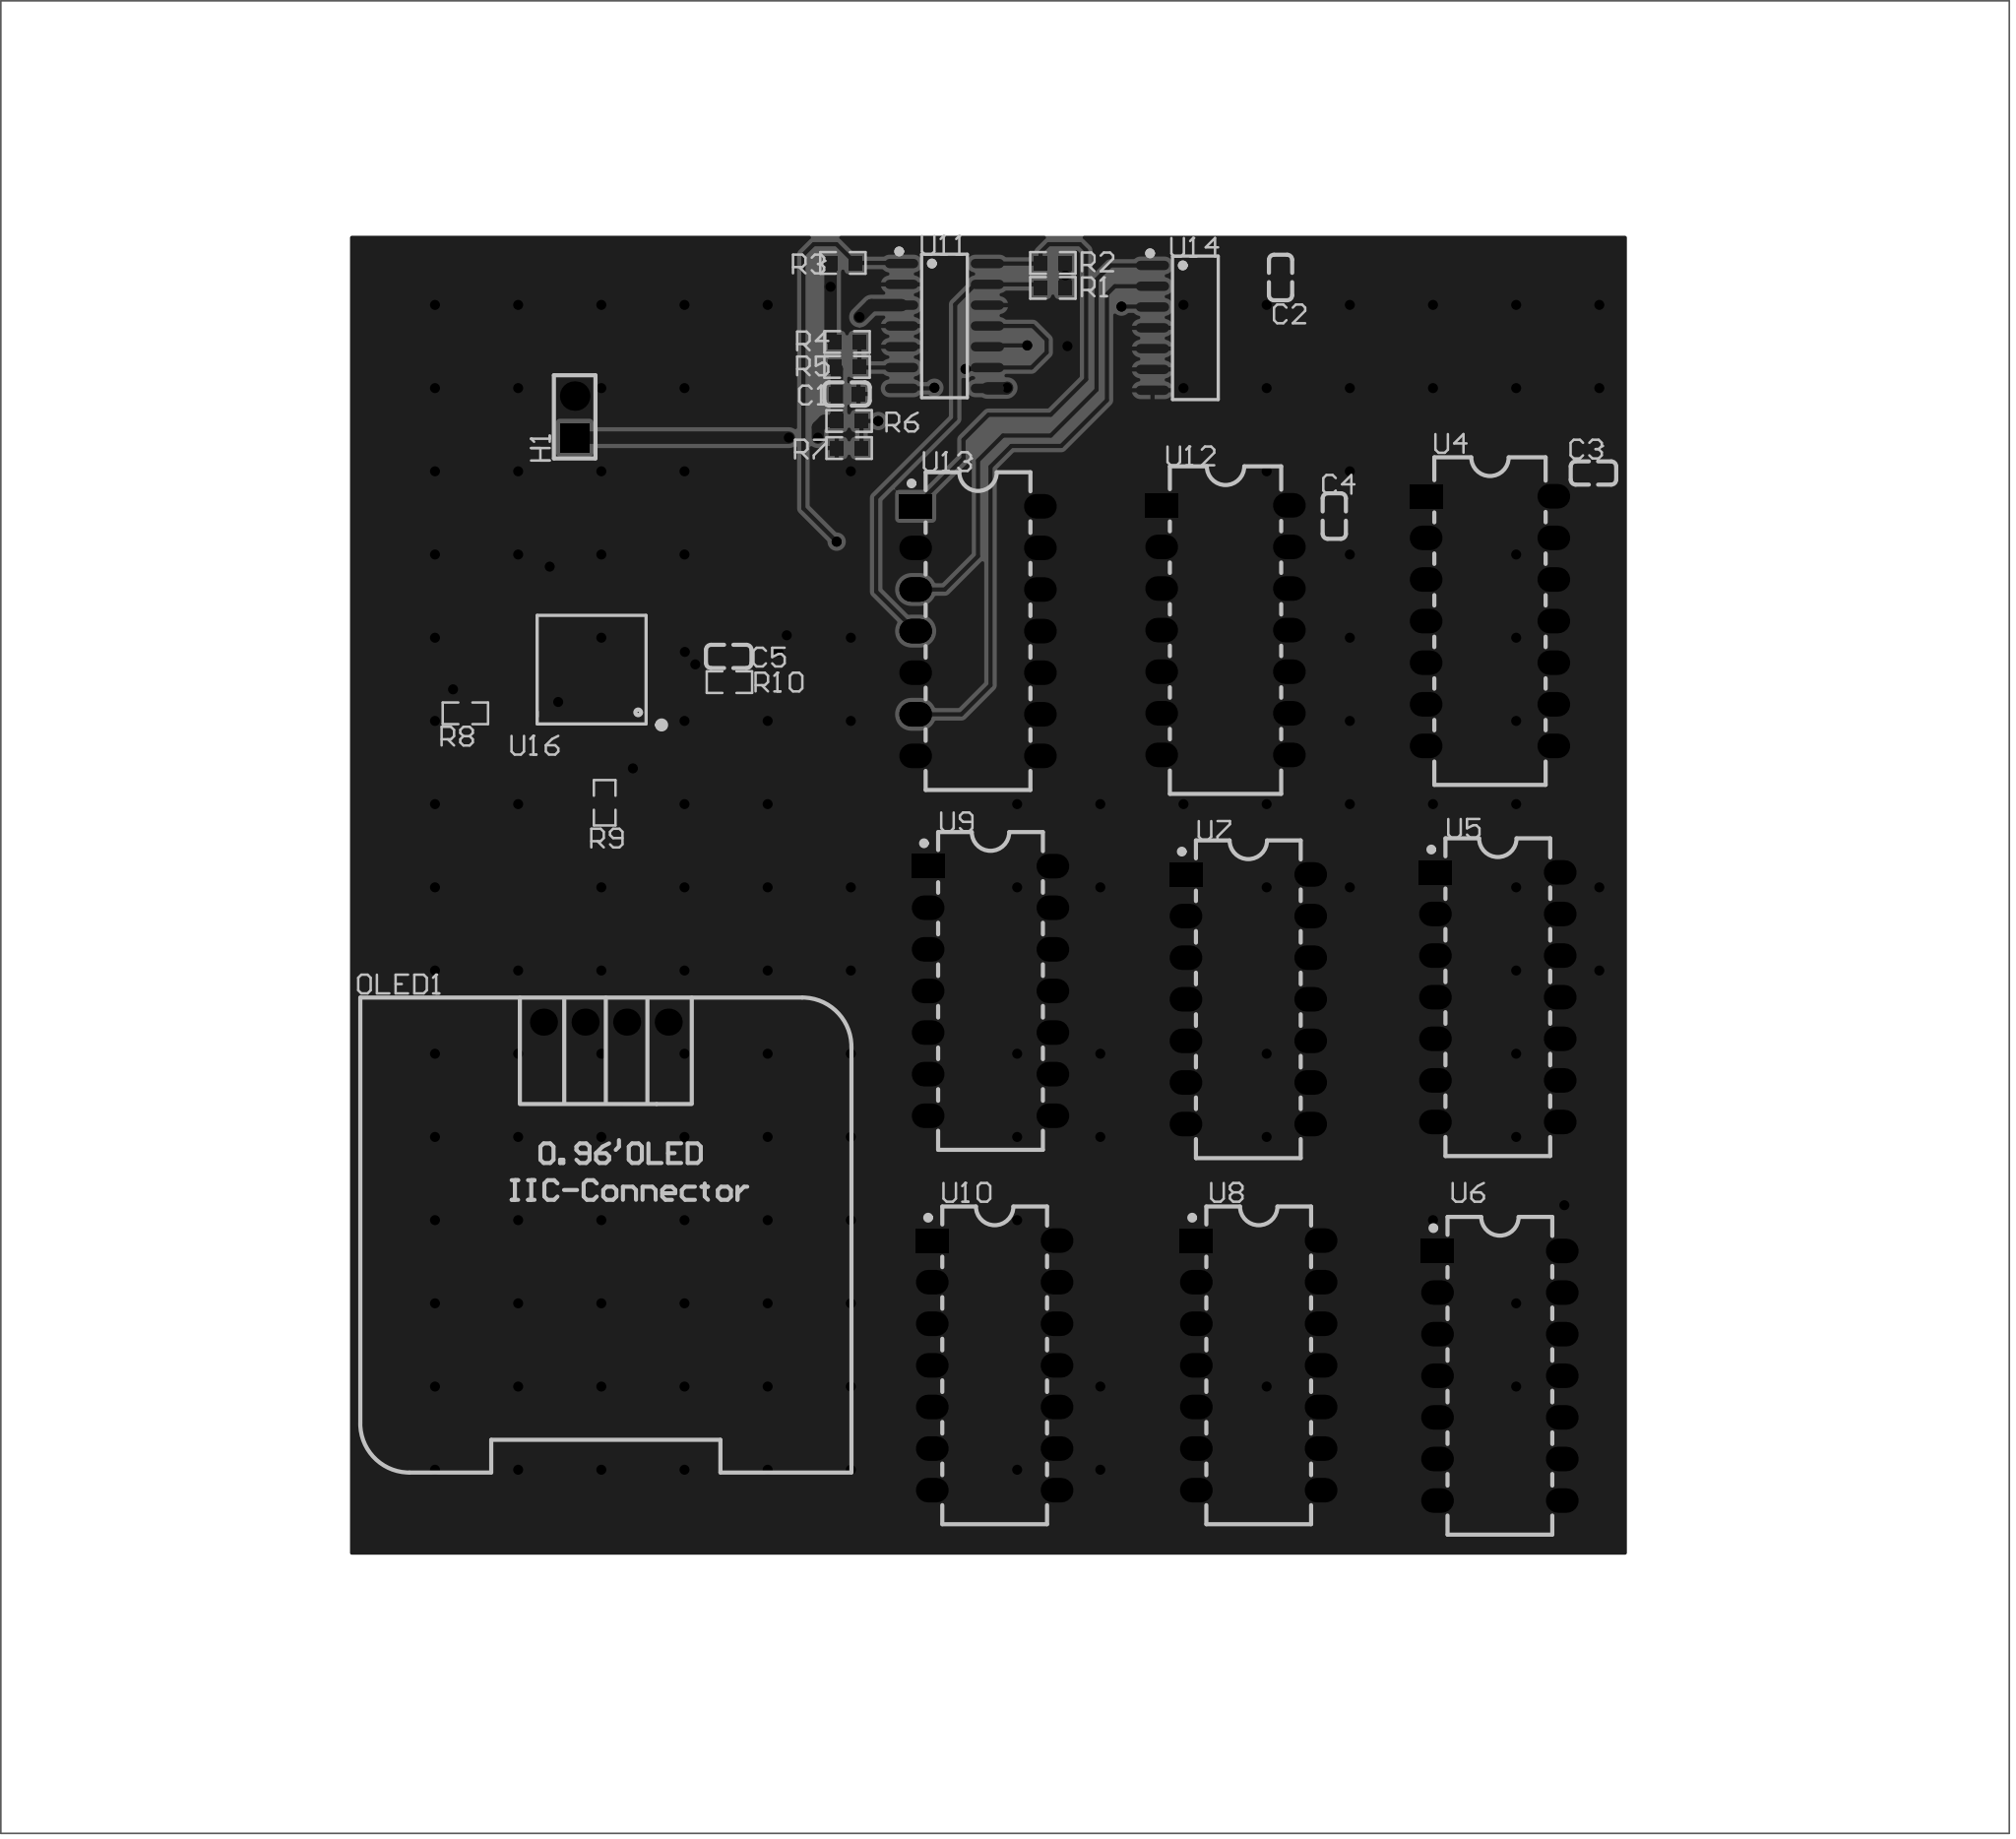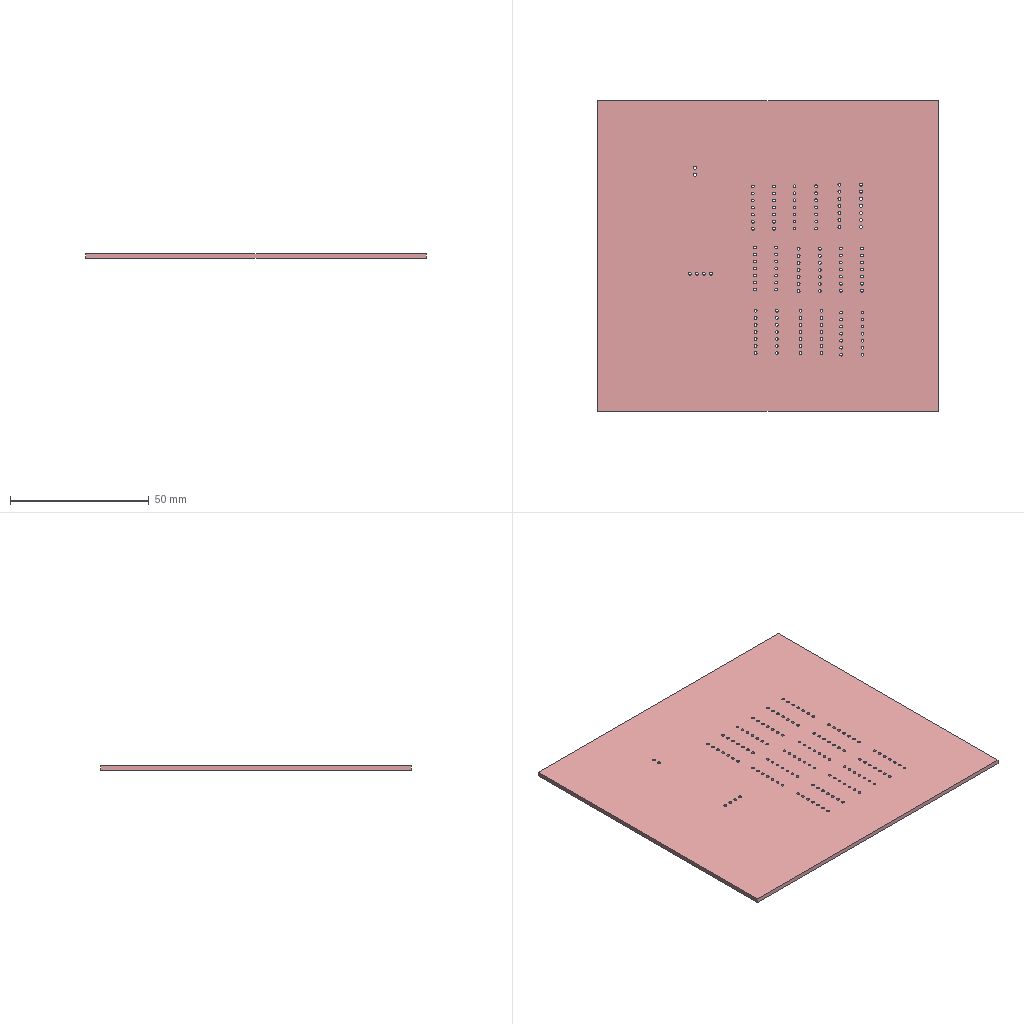Circuit board layout | Altium Designer | box 122.7 x 111.9 x 1.6 mm
Layer stack:
# Altium Designer layer stack of  (unit mm; dielectric type: 0 none, 1 core, 2 prepreg, 3 surface material)
index,name,kind,layer,copper_thickness_mm,dielectric_type,dielectric_thickness_mm,dielectric_material,dielectric_constant
0,Top Paste Mask Layer,other,,,,,,
1,Top Silkscreen Layer,other,,,,,,
2,Top Solder Mask Layer,dielectric,,,3,0.01,,3.3
3,Top Layer,copper,Top Layer,0.035,,,,
4,Dielectric1,dielectric,,,3,1.51,FR4,4.5
5,Bottom Layer,copper,Bottom Layer,0.035,,,,
6,Bottom Solder Mask Layer,dielectric,,,3,0.01,,3.3
7,Bottom Silkscreen Layer,other,,,,,,
8,Bottom Paste Mask Layer,other,,,,,,
# drill layer pairs: low layer,high layer
drill_pair,Top Layer,Bottom Layer
Part placement:
Designator,Comment,Layer,Footprint,Center-X(mm),Center-Y(mm),Rotation
C1,0.1u,TopLayer,C0603,121.539,157.734,180
C2,0.1u,TopLayer,C0603,148.019,164.845,90
C3,0.1u,TopLayer,C0603,167.132,152.908,180
C4,0.1u,TopLayer,C0603,151.3,150.279,90
C5,0.1u,TopLayer,C0603,114.311,141.71,180
OLED1,0.96OLED_4P,TopLayer,0.96OLED_4P,106.807,119.38,0
R1,10k,TopLayer,R0603,134.112,164.211,180
R2,1k,TopLayer,R0603,134.112,165.735,0
R3,1k,TopLayer,R0603,121.285,165.735,180
R4,2.2k,TopLayer,R0603,121.539,160.909,180
R5,2k,TopLayer,R0603,121.539,159.385,0
R6,100,TopLayer,R0603,121.666,156.083,180
R7,10,TopLayer,R0603,121.666,154.432,0
R8,10k,TopLayer,R0603,98.225,138.236,180
R9,10k,TopLayer,R0603,106.734,132.775,90
R10,10k,TopLayer,R0603,114.355,140.141,180
U4,74LS04DC,TopLayer,CDIP-14_L20.0-W6.8-P2.54-LS7.8-BL,160.81,143.867,270
U5,SN74LS11N,TopLayer,PDIP-14_L19.3-W6.4-P2.54-LS7.9-BL-1,161.29,120.904,270
U6,SN74LS11N,TopLayer,PDIP-14_L19.3-W6.4-P2.54-LS7.9-BL-1,161.417,97.79,270
U7,SN74LS11N,TopLayer,PDIP-14_L19.3-W6.4-P2.54-LS7.9-BL-1,146.05,120.777,270
U8,SN74LS11N,TopLayer,PDIP-14_L19.3-W6.4-P2.54-LS7.9-BL-1,146.685,98.425,270
U9,SN74LS11N,TopLayer,PDIP-14_L19.3-W6.4-P2.54-LS7.9-BL-1,130.302,121.285,270
U10,SN74LS11N,TopLayer,PDIP-14_L19.3-W6.4-P2.54-LS7.9-BL-1,130.556,98.425,270
U11,LM339D,TopLayer,SOIC-14_L8.7-W3.9-P1.27-LS6.0-BL,127.491,161.887,270
U12,74LS04DC,TopLayer,CDIP-14_L20.0-W6.8-P2.54-LS7.8-BL,144.658,143.317,270
U13,SN74LS08N,TopLayer,PDIP-14_L19.3-W6.4-P2.54-LS7.9-BL-1,129.54,143.256,270
U14,SN74LS32D,TopLayer,SOIC-14_L8.7-W3.9-P1.27-LS6.0-BL,142.816,161.772,270
U16,STM32F103C8T6,TopLayer,LQFP-48_L7.0-W7.0-P0.50-LS9.0-BL,105.95,140.915,90
H1,,TopLayer,HDR-TH_2P-P2.54-V-M-1,104.902,156.337,90
Pad and via stacks:
# Altium Designer via and pad stacks of  (unit mm). Each distinct definition once, with the count of objects using it.
# via: kind,start_layer,end_layer,hole_mm,diameter_mm,mode(0 simple;1 top-mid-bottom;2 full stack),diameter_per_layer,count,example_net
# pad: kind,layer,hole_mm,hole_type(0 round;1 square;2 slot),plating,top_size,top_shape(1 round;2 rect;3 octagon;9 rounded rect),mid_size,bottom_size,mode,footprint,size_per_layer,count,example
pad,Top Layer,0,0,plated,0.8x0.9,2,0.8x0.9,0.8x0.9,0,C0603,,10,C1.2
pad,Top Layer,0,0,plated,0.8065x0.864,2,0.8065x0.864,0.8065x0.864,0,R0603,,20,R1.2
pad,Top Layer,0,0,plated,0.574x2.038,1,0.574x2.038,0.574x2.038,0,SOIC-14_L8.7-W3.9-P1.27-LS6.0-BL,,28,U11.8
pad,Top Layer,0,0,plated,0.27x1.5,1,0.27x1.5,0.27x1.5,0,LQFP-48_L7.0-W7.0-P0.50-LS9.0-BL,,24,U16.1
pad,Top Layer,0,0,plated,1.5x0.27,1,1.5x0.27,1.5x0.27,0,LQFP-48_L7.0-W7.0-P0.50-LS9.0-BL,,24,U16.13
pad,Multi-Layer,1,0,plated,1.65x1.65,1,1.65x1.65,1.65x1.65,0,0.96OLED_4P,,4,OLED1.4
pad,Multi-Layer,1,0,plated,2x1.5,2,2x1.5,2x1.5,0,CDIP-14_L20.0-W6.8-P2.54-LS7.8-BL,,2,U4.1
pad,Multi-Layer,1,0,plated,2x1.5,1,2x1.5,2x1.5,0,CDIP-14_L20.0-W6.8-P2.54-LS7.8-BL,,26,U4.2
pad,Multi-Layer,1,0,plated,2x1.5,2,2x1.5,2x1.5,0,PDIP-14_L19.3-W6.4-P2.54-LS7.9-BL-1,,7,U5.1
pad,Multi-Layer,1,0,plated,2x1.5,1,2x1.5,2x1.5,0,PDIP-14_L19.3-W6.4-P2.54-LS7.9-BL-1,,91,U5.2
pad,Multi-Layer,1.1,0,plated,1.8x1.8,1,1.8x1.8,1.8x1.8,0,HDR-TH_2P-P2.54-V-M-1,,1,H1.2
pad,Multi-Layer,1.1,0,plated,1.8x1.8,2,1.8x1.8,1.8x1.8,0,HDR-TH_2P-P2.54-V-M-1,,1,H1.1
via,Top Layer,Bottom Layer,0.3048,0.61,0,,149,$4N3
Copper pours:
name,layer,net,type(0 solid;1 hatched;2 none)
Bottom Layer-GND,Bottom Layer,GND,0
Top Layer-GND,Top Layer,GND,0